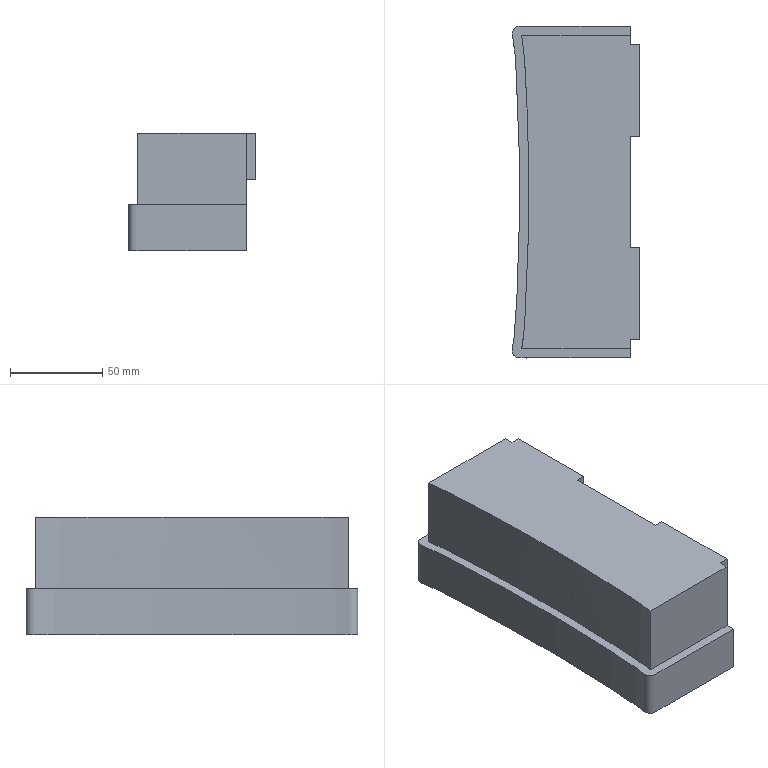Part | NX | features solid 2 | 1 solid | 28 faces | box 69.104 x 180.06 x 64 mm | volume 482191 mm3 | plane 19 | spline 5 | cylinder 4 | commonest cylinder face diameters 20 x2 30 x2
STEP:
#1=CARTESIAN_POINT('',(770.,80.,130.));
#2=VERTEX_POINT('',#1);
#3=CARTESIAN_POINT('',(770.,85.,130.));
#4=VERTEX_POINT('',#3);
#5=CARTESIAN_POINT('',(770.,120.,130.));
#6=DIRECTION('',(0.,-1.,0.));
#7=VECTOR('',#6,1000.);
#8=LINE('',#5,#7);
#9=EDGE_CURVE('',#2,#4,#8,.F.);
#10=ORIENTED_EDGE('',*,*,#9,.F.);
#11=CARTESIAN_POINT('',(770.,80.,105.));
#12=VERTEX_POINT('',#11);
#13=CARTESIAN_POINT('',(770.,80.,130.));
#14=DIRECTION('',(0.,0.,1.));
#15=VECTOR('',#14,1000.);
#16=LINE('',#13,#15);
#17=EDGE_CURVE('',#2,#12,#16,.F.);
#18=ORIENTED_EDGE('',*,*,#17,.T.);
#19=CARTESIAN_POINT('',(770.,65.,105.));
#20=VERTEX_POINT('',#19);
#21=CARTESIAN_POINT('',(770.,50.,105.));
#22=DIRECTION('',(0.,1.,0.));
#23=VECTOR('',#22,1000.);
#24=LINE('',#21,#23);
#25=EDGE_CURVE('',#12,#20,#24,.F.);
#26=ORIENTED_EDGE('',*,*,#25,.T.);
#27=CARTESIAN_POINT('',(770.,65.,66.));
#28=VERTEX_POINT('',#27);
#29=CARTESIAN_POINT('',(770.,65.,50.));
#30=DIRECTION('',(0.,0.,-1.));
#31=VECTOR('',#30,1000.);
#32=LINE('',#29,#31);
#33=EDGE_CURVE('',#28,#20,#32,.F.);
#34=ORIENTED_EDGE('',*,*,#33,.F.);
#35=CARTESIAN_POINT('',(770.,90.,66.));
#36=VERTEX_POINT('',#35);
#37=CARTESIAN_POINT('',(770.,120.,66.));
#38=DIRECTION('',(0.,1.,0.));
#39=VECTOR('',#38,1000.);
#40=LINE('',#37,#39);
#41=EDGE_CURVE('',#36,#28,#40,.F.);
#42=ORIENTED_EDGE('',*,*,#41,.F.);
#43=CARTESIAN_POINT('',(770.,90.,91.));
#44=VERTEX_POINT('',#43);
#45=CARTESIAN_POINT('',(770.,90.,98.));
#46=DIRECTION('',(0.,0.,1.));
#47=VECTOR('',#46,1000.);
#48=LINE('',#45,#47);
#49=EDGE_CURVE('',#36,#44,#48,.T.);
#50=ORIENTED_EDGE('',*,*,#49,.T.);
#51=CARTESIAN_POINT('',(770.,85.,91.));
#52=VERTEX_POINT('',#51);
#53=CARTESIAN_POINT('',(770.,90.,91.));
#54=DIRECTION('',(0.,-1.,0.));
#55=VECTOR('',#54,1000.);
#56=LINE('',#53,#55);
#57=EDGE_CURVE('',#44,#52,#56,.T.);
#58=ORIENTED_EDGE('',*,*,#57,.T.);
#59=CARTESIAN_POINT('',(770.,85.,91.));
#60=DIRECTION('',(0.,0.,1.));
#61=VECTOR('',#60,1000.);
#62=LINE('',#59,#61);
#63=EDGE_CURVE('',#52,#4,#62,.T.);
#64=ORIENTED_EDGE('',*,*,#63,.T.);
#65=EDGE_LOOP('',(#10,#18,#26,#34,#42,#50,#58,#64));
#66=FACE_BOUND('',#65,.T.);
#67=CARTESIAN_POINT('',(770.,120.,50.));
#68=DIRECTION('',(1.,0.,0.));
#69=DIRECTION('',(0.,0.,-1.));
#70=AXIS2_PLACEMENT_3D('',#67,#68,#69);
#71=PLANE('',#70);
#72=ADVANCED_FACE('',(#66),#71,.T.);
#73=CARTESIAN_POINT('',(770.,30.,105.));
#74=VERTEX_POINT('',#73);
#75=CARTESIAN_POINT('',(770.,-30.,105.));
#76=VERTEX_POINT('',#75);
#77=CARTESIAN_POINT('',(770.,120.,105.));
#78=DIRECTION('',(0.,1.,0.));
#79=VECTOR('',#78,1000.);
#80=LINE('',#77,#79);
#81=EDGE_CURVE('',#74,#76,#80,.F.);
#82=ORIENTED_EDGE('',*,*,#81,.F.);
#83=CARTESIAN_POINT('',(770.,30.,130.));
#84=VERTEX_POINT('',#83);
#85=CARTESIAN_POINT('',(770.,30.,130.));
#86=DIRECTION('',(0.,0.,-1.));
#87=VECTOR('',#86,1000.);
#88=LINE('',#85,#87);
#89=EDGE_CURVE('',#84,#74,#88,.T.);
#90=ORIENTED_EDGE('',*,*,#89,.F.);
#91=CARTESIAN_POINT('',(770.,-30.,130.));
#92=VERTEX_POINT('',#91);
#93=CARTESIAN_POINT('',(770.,120.,130.));
#94=DIRECTION('',(0.,-1.,0.));
#95=VECTOR('',#94,1000.);
#96=LINE('',#93,#95);
#97=EDGE_CURVE('',#92,#84,#96,.F.);
#98=ORIENTED_EDGE('',*,*,#97,.F.);
#99=CARTESIAN_POINT('',(770.,-30.,130.));
#100=DIRECTION('',(0.,0.,-1.));
#101=VECTOR('',#100,1000.);
#102=LINE('',#99,#101);
#103=EDGE_CURVE('',#92,#76,#102,.T.);
#104=ORIENTED_EDGE('',*,*,#103,.T.);
#105=EDGE_LOOP('',(#82,#90,#98,#104));
#106=FACE_BOUND('',#105,.T.);
#107=CARTESIAN_POINT('',(770.,120.,50.));
#108=DIRECTION('',(1.,0.,0.));
#109=DIRECTION('',(0.,0.,-1.));
#110=AXIS2_PLACEMENT_3D('',#107,#108,#109);
#111=PLANE('',#110);
#112=ADVANCED_FACE('',(#106),#111,.T.);
#113=CARTESIAN_POINT('',(711.016,85.028,130.));
#114=VERTEX_POINT('',#113);
#115=CARTESIAN_POINT('',(711.009,-85.029,130.));
#116=VERTEX_POINT('',#115);
#117=CARTESIAN_POINT('',(711.016,85.028,130.));
#118=CARTESIAN_POINT('',(711.113,84.38,130.));
#119=CARTESIAN_POINT('',(711.28,83.237,130.));
#120=CARTESIAN_POINT('',(711.512,81.583,130.));
#121=CARTESIAN_POINT('',(711.653,80.568,130.));
#122=CARTESIAN_POINT('',(711.81,79.426,130.));
#123=CARTESIAN_POINT('',(711.951,78.38,130.));
#124=CARTESIAN_POINT('',(712.186,76.65,130.));
#125=CARTESIAN_POINT('',(712.426,74.446,130.));
#126=CARTESIAN_POINT('',(712.563,71.77,130.));
#127=CARTESIAN_POINT('',(712.789,68.223,130.));
#128=CARTESIAN_POINT('',(713.036,63.843,130.));
#129=CARTESIAN_POINT('',(713.326,58.444,130.));
#130=CARTESIAN_POINT('',(713.587,53.129,130.));
#131=CARTESIAN_POINT('',(713.826,47.81,130.));
#132=CARTESIAN_POINT('',(714.036,42.612,130.));
#133=CARTESIAN_POINT('',(714.234,37.124,130.));
#134=CARTESIAN_POINT('',(714.457,29.957,130.));
#135=CARTESIAN_POINT('',(714.674,21.033,130.));
#136=CARTESIAN_POINT('',(714.828,10.445,130.));
#137=CARTESIAN_POINT('',(714.895,-3.481,130.));
#138=CARTESIAN_POINT('',(714.754,-17.426,130.));
#139=CARTESIAN_POINT('',(714.447,-29.939,130.));
#140=CARTESIAN_POINT('',(714.221,-37.113,130.));
#141=CARTESIAN_POINT('',(714.022,-42.617,130.));
#142=CARTESIAN_POINT('',(713.812,-47.802,130.));
#143=CARTESIAN_POINT('',(713.573,-53.121,130.));
#144=CARTESIAN_POINT('',(713.312,-58.436,130.));
#145=CARTESIAN_POINT('',(713.023,-63.845,130.));
#146=CARTESIAN_POINT('',(712.772,-68.224,130.));
#147=CARTESIAN_POINT('',(712.585,-71.32,130.));
#148=CARTESIAN_POINT('',(712.487,-72.892,130.));
#149=CARTESIAN_POINT('',(712.433,-73.755,130.));
#150=CARTESIAN_POINT('',(712.387,-74.507,130.));
#151=CARTESIAN_POINT('',(712.36,-74.864,130.));
#152=CARTESIAN_POINT('',(712.291,-75.607,130.));
#153=CARTESIAN_POINT('',(712.173,-76.66,130.));
#154=CARTESIAN_POINT('',(711.96,-78.303,130.));
#155=CARTESIAN_POINT('',(711.632,-80.652,130.));
#156=CARTESIAN_POINT('',(711.306,-82.996,130.));
#157=CARTESIAN_POINT('',(711.097,-84.435,130.));
#158=CARTESIAN_POINT('',(711.009,-85.029,130.));
#159=B_SPLINE_CURVE_WITH_KNOTS('',3,(#117,#118,#119,#120,#121,#122,#123,#124,#125,#126,#127,#128,#129,#130,#131,#132,#133,#134,#135,#136,#137,#138,#139,#140,#141,#142,#143,#144,#145,#146,#147,#148,#149,#150,#151,#152,#153,#154,#155,#156,#157,#158),.UNSPECIFIED.,.F.,.F.,(4,1,1,1,1,1,1,1,1,1,1,1,1,1,1,1,1,1,1,1,1,1,1,1,1,1,1,1,1,1,1,1,1,1,1,1,1,1,1,4),(0.,0.01562,0.02344,0.02734,0.03125,0.03906,0.04688,0.0625,0.07812,0.09375,0.125,0.1562,0.1875,0.2188,0.25,0.2812,0.3125,0.375,0.4375,0.5,0.625,0.6875,0.7188,0.75,0.7812,0.8125,0.8438,0.875,0.9062,0.9219,0.9297,0.9336,0.9375,0.9414,0.9453,0.9531,0.9609,0.9688,0.9844,1.),.UNSPECIFIED.);
#160=EDGE_CURVE('',#114,#116,#159,.T.);
#161=ORIENTED_EDGE('',*,*,#160,.T.);
#162=CARTESIAN_POINT('',(770.,-85.,130.));
#163=VERTEX_POINT('',#162);
#164=CARTESIAN_POINT('',(711.009,-85.029,130.));
#165=CARTESIAN_POINT('',(717.1,-85.01,130.));
#166=CARTESIAN_POINT('',(736.764,-85.,130.));
#167=CARTESIAN_POINT('',(770.,-85.,130.));
#168=B_SPLINE_CURVE_WITH_KNOTS('',3,(#164,#165,#166,#167),.UNSPECIFIED.,.F.,.F.,(4,4),(0.,1.),.UNSPECIFIED.);
#169=EDGE_CURVE('',#116,#163,#168,.T.);
#170=ORIENTED_EDGE('',*,*,#169,.T.);
#171=CARTESIAN_POINT('',(770.,-80.,130.));
#172=VERTEX_POINT('',#171);
#173=CARTESIAN_POINT('',(770.,120.,130.));
#174=DIRECTION('',(0.,-1.,0.));
#175=VECTOR('',#174,1000.);
#176=LINE('',#173,#175);
#177=EDGE_CURVE('',#163,#172,#176,.F.);
#178=ORIENTED_EDGE('',*,*,#177,.T.);
#179=CARTESIAN_POINT('',(775.,-80.,130.));
#180=VERTEX_POINT('',#179);
#181=CARTESIAN_POINT('',(775.,-80.,130.));
#182=DIRECTION('',(-1.,0.,0.));
#183=VECTOR('',#182,1000.);
#184=LINE('',#181,#183);
#185=EDGE_CURVE('',#180,#172,#184,.T.);
#186=ORIENTED_EDGE('',*,*,#185,.F.);
#187=CARTESIAN_POINT('',(775.,-30.,130.));
#188=VERTEX_POINT('',#187);
#189=CARTESIAN_POINT('',(775.,-90.,130.));
#190=DIRECTION('',(0.,1.,0.));
#191=VECTOR('',#190,1000.);
#192=LINE('',#189,#191);
#193=EDGE_CURVE('',#180,#188,#192,.T.);
#194=ORIENTED_EDGE('',*,*,#193,.T.);
#195=CARTESIAN_POINT('',(775.,-30.,130.));
#196=DIRECTION('',(-1.,0.,0.));
#197=VECTOR('',#196,1000.);
#198=LINE('',#195,#197);
#199=EDGE_CURVE('',#188,#92,#198,.T.);
#200=ORIENTED_EDGE('',*,*,#199,.T.);
#201=ORIENTED_EDGE('',*,*,#97,.T.);
#202=CARTESIAN_POINT('',(775.,30.,130.));
#203=VERTEX_POINT('',#202);
#204=CARTESIAN_POINT('',(775.,30.,130.));
#205=DIRECTION('',(-1.,0.,0.));
#206=VECTOR('',#205,1000.);
#207=LINE('',#204,#206);
#208=EDGE_CURVE('',#203,#84,#207,.T.);
#209=ORIENTED_EDGE('',*,*,#208,.F.);
#210=CARTESIAN_POINT('',(775.,80.,130.));
#211=VERTEX_POINT('',#210);
#212=CARTESIAN_POINT('',(775.,50.,130.));
#213=DIRECTION('',(0.,-1.,0.));
#214=VECTOR('',#213,1000.);
#215=LINE('',#212,#214);
#216=EDGE_CURVE('',#211,#203,#215,.T.);
#217=ORIENTED_EDGE('',*,*,#216,.F.);
#218=CARTESIAN_POINT('',(775.,80.,130.));
#219=DIRECTION('',(1.,0.,0.));
#220=VECTOR('',#219,1000.);
#221=LINE('',#218,#220);
#222=EDGE_CURVE('',#211,#2,#221,.F.);
#223=ORIENTED_EDGE('',*,*,#222,.T.);
#224=ORIENTED_EDGE('',*,*,#9,.T.);
#225=CARTESIAN_POINT('',(770.,85.,130.));
#226=CARTESIAN_POINT('',(735.052,85.,130.));
#227=CARTESIAN_POINT('',(715.391,85.009,130.));
#228=CARTESIAN_POINT('',(711.016,85.028,130.));
#229=B_SPLINE_CURVE_WITH_KNOTS('',3,(#225,#226,#227,#228),.UNSPECIFIED.,.F.,.F.,(4,4),(0.,1.),.UNSPECIFIED.);
#230=EDGE_CURVE('',#4,#114,#229,.T.);
#231=ORIENTED_EDGE('',*,*,#230,.T.);
#232=EDGE_LOOP('',(#161,#170,#178,#186,#194,#200,#201,#209,#217,#223,#224,#231));
#233=FACE_BOUND('',#232,.T.);
#234=CARTESIAN_POINT('',(0.,0.,130.));
#235=DIRECTION('',(0.,0.,1.));
#236=DIRECTION('',(1.,0.,0.));
#237=AXIS2_PLACEMENT_3D('',#234,#235,#236);
#238=PLANE('',#237);
#239=ADVANCED_FACE('',(#233),#238,.T.);
#240=CARTESIAN_POINT('',(770.,-90.,91.));
#241=VERTEX_POINT('',#240);
#242=CARTESIAN_POINT('',(770.,-90.,66.));
#243=VERTEX_POINT('',#242);
#244=CARTESIAN_POINT('',(770.,-90.,98.));
#245=DIRECTION('',(0.,0.,1.));
#246=VECTOR('',#245,1000.);
#247=LINE('',#244,#246);
#248=EDGE_CURVE('',#241,#243,#247,.F.);
#249=ORIENTED_EDGE('',*,*,#248,.F.);
#250=CARTESIAN_POINT('',(790.,-90.,91.));
#251=CARTESIAN_POINT('',(782.313,-90.,91.));
#252=CARTESIAN_POINT('',(774.625,-90.,91.));
#253=CARTESIAN_POINT('',(766.938,-90.,91.));
#254=CARTESIAN_POINT('',(757.429,-90.,91.));
#255=CARTESIAN_POINT('',(738.707,-90.,91.));
#256=CARTESIAN_POINT('',(719.689,-90.,91.));
#257=CARTESIAN_POINT('',(709.611,-90.034,91.));
#258=CARTESIAN_POINT('',(708.18,-89.742,91.));
#259=CARTESIAN_POINT('',(706.773,-88.715,91.));
#260=CARTESIAN_POINT('',(705.945,-87.182,91.));
#261=CARTESIAN_POINT('',(705.849,-85.71,91.));
#262=CARTESIAN_POINT('',(706.186,-83.502,91.));
#263=CARTESIAN_POINT('',(706.636,-80.205,91.));
#264=CARTESIAN_POINT('',(707.096,-77.043,91.));
#265=CARTESIAN_POINT('',(707.332,-75.034,91.));
#266=CARTESIAN_POINT('',(707.37,-74.599,91.));
#267=CARTESIAN_POINT('',(708.17,-62.019,91.));
#268=CARTESIAN_POINT('',(709.408,-37.195,91.));
#269=CARTESIAN_POINT('',(710.084,-0.0009582,91.));
#270=CARTESIAN_POINT('',(709.422,37.194,91.));
#271=CARTESIAN_POINT('',(708.185,62.018,91.));
#272=CARTESIAN_POINT('',(707.381,74.598,91.));
#273=CARTESIAN_POINT('',(707.346,75.035,91.));
#274=CARTESIAN_POINT('',(707.091,77.042,91.));
#275=CARTESIAN_POINT('',(706.658,80.207,91.));
#276=CARTESIAN_POINT('',(706.194,83.501,91.));
#277=CARTESIAN_POINT('',(705.854,85.708,91.));
#278=CARTESIAN_POINT('',(705.949,87.18,91.));
#279=CARTESIAN_POINT('',(706.777,88.714,91.));
#280=CARTESIAN_POINT('',(708.184,89.742,91.));
#281=CARTESIAN_POINT('',(709.621,90.034,91.));
#282=CARTESIAN_POINT('',(717.126,90.,91.));
#283=CARTESIAN_POINT('',(730.996,90.,91.));
#284=CARTESIAN_POINT('',(744.562,90.,91.));
#285=CARTESIAN_POINT('',(751.497,90.,91.));
#286=CARTESIAN_POINT('',(764.331,90.,91.));
#287=CARTESIAN_POINT('',(777.166,90.,91.));
#288=CARTESIAN_POINT('',(790.,90.,91.));
#289=B_SPLINE_CURVE_WITH_KNOTS('',3,(#250,#251,#252,#253,#254,#255,#256,#257,#258,#259,#260,#261,#262,#263,#264,#265,#266,#267,#268,#269,#270,#271,#272,#273,#274,#275,#276,#277,#278,#279,#280,#281,#282,#283,#284,#285,#286,#287,#288),.UNSPECIFIED.,.F.,.F.,(4,3,1,1,1,1,1,1,1,1,1,1,1,1,1,1,1,1,1,1,1,1,1,1,1,1,1,1,1,1,1,3,4),(-0.08134,0.,0.1006,0.1981,0.2012,0.2072,0.2133,0.2193,0.2253,0.2286,0.2429,0.2605,0.2624,0.2643,0.2651,0.3958,0.5272,0.6587,0.7893,0.7902,0.7921,0.794,0.8116,0.8259,0.8292,0.8352,0.8412,0.8472,0.8532,0.8565,0.9266,1.,1.136),.UNSPECIFIED.);
#290=EDGE_CURVE('',#241,#44,#289,.T.);
#291=ORIENTED_EDGE('',*,*,#290,.T.);
#292=ORIENTED_EDGE('',*,*,#49,.F.);
#293=CARTESIAN_POINT('',(809.468,-90.,66.));
#294=CARTESIAN_POINT('',(795.291,-90.,66.));
#295=CARTESIAN_POINT('',(781.115,-90.,66.));
#296=CARTESIAN_POINT('',(766.938,-90.,66.));
#297=CARTESIAN_POINT('',(757.429,-90.,66.));
#298=CARTESIAN_POINT('',(738.707,-90.,66.));
#299=CARTESIAN_POINT('',(719.689,-90.,66.));
#300=CARTESIAN_POINT('',(709.611,-90.034,66.));
#301=CARTESIAN_POINT('',(708.18,-89.742,66.));
#302=CARTESIAN_POINT('',(706.773,-88.715,66.));
#303=CARTESIAN_POINT('',(705.945,-87.182,66.));
#304=CARTESIAN_POINT('',(705.849,-85.71,66.));
#305=CARTESIAN_POINT('',(706.186,-83.502,66.));
#306=CARTESIAN_POINT('',(706.636,-80.205,66.));
#307=CARTESIAN_POINT('',(707.096,-77.043,66.));
#308=CARTESIAN_POINT('',(707.332,-75.034,66.));
#309=CARTESIAN_POINT('',(707.37,-74.599,66.));
#310=CARTESIAN_POINT('',(708.17,-62.019,66.));
#311=CARTESIAN_POINT('',(709.408,-37.195,66.));
#312=CARTESIAN_POINT('',(710.084,-0.0009582,66.));
#313=CARTESIAN_POINT('',(709.422,37.194,66.));
#314=CARTESIAN_POINT('',(708.185,62.018,66.));
#315=CARTESIAN_POINT('',(707.381,74.598,66.));
#316=CARTESIAN_POINT('',(707.346,75.035,66.));
#317=CARTESIAN_POINT('',(707.091,77.042,66.));
#318=CARTESIAN_POINT('',(706.658,80.207,66.));
#319=CARTESIAN_POINT('',(706.194,83.501,66.));
#320=CARTESIAN_POINT('',(705.854,85.708,66.));
#321=CARTESIAN_POINT('',(705.949,87.18,66.));
#322=CARTESIAN_POINT('',(706.777,88.714,66.));
#323=CARTESIAN_POINT('',(708.184,89.742,66.));
#324=CARTESIAN_POINT('',(709.621,90.034,66.));
#325=CARTESIAN_POINT('',(717.126,90.,66.));
#326=CARTESIAN_POINT('',(730.996,90.,66.));
#327=CARTESIAN_POINT('',(744.562,90.,66.));
#328=CARTESIAN_POINT('',(751.497,90.,66.));
#329=CARTESIAN_POINT('',(765.674,90.,66.));
#330=CARTESIAN_POINT('',(779.851,90.,66.));
#331=CARTESIAN_POINT('',(794.028,90.,66.));
#332=B_SPLINE_CURVE_WITH_KNOTS('',3,(#293,#294,#295,#296,#297,#298,#299,#300,#301,#302,#303,#304,#305,#306,#307,#308,#309,#310,#311,#312,#313,#314,#315,#316,#317,#318,#319,#320,#321,#322,#323,#324,#325,#326,#327,#328,#329,#330,#331),.UNSPECIFIED.,.F.,.F.,(4,3,1,1,1,1,1,1,1,1,1,1,1,1,1,1,1,1,1,1,1,1,1,1,1,1,1,1,1,1,1,3,4),(-0.15,0.,0.1006,0.1981,0.2012,0.2072,0.2133,0.2193,0.2253,0.2286,0.2429,0.2605,0.2624,0.2643,0.2651,0.3958,0.5272,0.6587,0.7893,0.7902,0.7921,0.794,0.8116,0.8259,0.8292,0.8352,0.8412,0.8472,0.8532,0.8565,0.9266,1.,1.15),.UNSPECIFIED.);
#333=EDGE_CURVE('',#36,#243,#332,.F.);
#334=ORIENTED_EDGE('',*,*,#333,.T.);
#335=EDGE_LOOP('',(#249,#291,#292,#334));
#336=FACE_BOUND('',#335,.T.);
#337=CARTESIAN_POINT('',(770.,-90.,66.));
#338=CARTESIAN_POINT('',(770.,-90.,91.));
#339=CARTESIAN_POINT('',(768.979,-90.,66.));
#340=CARTESIAN_POINT('',(768.979,-90.,91.));
#341=CARTESIAN_POINT('',(767.958,-90.,66.));
#342=CARTESIAN_POINT('',(767.958,-90.,91.));
#343=CARTESIAN_POINT('',(766.938,-90.,66.));
#344=CARTESIAN_POINT('',(766.938,-90.,91.));
#345=CARTESIAN_POINT('',(757.429,-90.,66.));
#346=CARTESIAN_POINT('',(757.429,-90.,91.));
#347=CARTESIAN_POINT('',(738.707,-90.,66.));
#348=CARTESIAN_POINT('',(738.707,-90.,91.));
#349=CARTESIAN_POINT('',(719.689,-90.,66.));
#350=CARTESIAN_POINT('',(719.689,-90.,91.));
#351=CARTESIAN_POINT('',(709.611,-90.034,66.));
#352=CARTESIAN_POINT('',(709.611,-90.034,91.));
#353=CARTESIAN_POINT('',(708.18,-89.742,66.));
#354=CARTESIAN_POINT('',(708.18,-89.742,91.));
#355=CARTESIAN_POINT('',(706.773,-88.715,66.));
#356=CARTESIAN_POINT('',(706.773,-88.715,91.));
#357=CARTESIAN_POINT('',(705.945,-87.182,66.));
#358=CARTESIAN_POINT('',(705.945,-87.182,91.));
#359=CARTESIAN_POINT('',(705.849,-85.71,66.));
#360=CARTESIAN_POINT('',(705.849,-85.71,91.));
#361=CARTESIAN_POINT('',(706.186,-83.502,66.));
#362=CARTESIAN_POINT('',(706.186,-83.502,91.));
#363=CARTESIAN_POINT('',(706.636,-80.205,66.));
#364=CARTESIAN_POINT('',(706.636,-80.205,91.));
#365=CARTESIAN_POINT('',(707.096,-77.043,66.));
#366=CARTESIAN_POINT('',(707.096,-77.043,91.));
#367=CARTESIAN_POINT('',(707.332,-75.034,66.));
#368=CARTESIAN_POINT('',(707.332,-75.034,91.));
#369=CARTESIAN_POINT('',(707.37,-74.599,66.));
#370=CARTESIAN_POINT('',(707.37,-74.599,91.));
#371=CARTESIAN_POINT('',(708.17,-62.019,66.));
#372=CARTESIAN_POINT('',(708.17,-62.019,91.));
#373=CARTESIAN_POINT('',(709.408,-37.195,66.));
#374=CARTESIAN_POINT('',(709.408,-37.195,91.));
#375=CARTESIAN_POINT('',(710.084,-0.0009582,66.));
#376=CARTESIAN_POINT('',(710.084,-0.0009582,91.));
#377=CARTESIAN_POINT('',(709.422,37.194,66.));
#378=CARTESIAN_POINT('',(709.422,37.194,91.));
#379=CARTESIAN_POINT('',(708.185,62.018,66.));
#380=CARTESIAN_POINT('',(708.185,62.018,91.));
#381=CARTESIAN_POINT('',(707.381,74.598,66.));
#382=CARTESIAN_POINT('',(707.381,74.598,91.));
#383=CARTESIAN_POINT('',(707.346,75.035,66.));
#384=CARTESIAN_POINT('',(707.346,75.035,91.));
#385=CARTESIAN_POINT('',(707.091,77.042,66.));
#386=CARTESIAN_POINT('',(707.091,77.042,91.));
#387=CARTESIAN_POINT('',(706.658,80.207,66.));
#388=CARTESIAN_POINT('',(706.658,80.207,91.));
#389=CARTESIAN_POINT('',(706.194,83.501,66.));
#390=CARTESIAN_POINT('',(706.194,83.501,91.));
#391=CARTESIAN_POINT('',(705.854,85.708,66.));
#392=CARTESIAN_POINT('',(705.854,85.708,91.));
#393=CARTESIAN_POINT('',(705.949,87.18,66.));
#394=CARTESIAN_POINT('',(705.949,87.18,91.));
#395=CARTESIAN_POINT('',(706.777,88.714,66.));
#396=CARTESIAN_POINT('',(706.777,88.714,91.));
#397=CARTESIAN_POINT('',(708.184,89.742,66.));
#398=CARTESIAN_POINT('',(708.184,89.742,91.));
#399=CARTESIAN_POINT('',(709.621,90.034,66.));
#400=CARTESIAN_POINT('',(709.621,90.034,91.));
#401=CARTESIAN_POINT('',(717.126,90.,66.));
#402=CARTESIAN_POINT('',(717.126,90.,91.));
#403=CARTESIAN_POINT('',(730.996,90.,66.));
#404=CARTESIAN_POINT('',(730.996,90.,91.));
#405=CARTESIAN_POINT('',(744.562,90.,66.));
#406=CARTESIAN_POINT('',(744.562,90.,91.));
#407=CARTESIAN_POINT('',(751.497,90.,66.));
#408=CARTESIAN_POINT('',(751.497,90.,91.));
#409=CARTESIAN_POINT('',(757.665,90.,66.));
#410=CARTESIAN_POINT('',(757.665,90.,91.));
#411=CARTESIAN_POINT('',(763.832,90.,66.));
#412=CARTESIAN_POINT('',(763.832,90.,91.));
#413=CARTESIAN_POINT('',(770.,90.,66.));
#414=CARTESIAN_POINT('',(770.,90.,91.));
#415=B_SPLINE_SURFACE_WITH_KNOTS('',3,1,((#337,#338),(#339,#340),(#341,#342),(#343,#344),(#345,#346),(#347,#348),(#349,#350),(#351,#352),(#353,#354),(#355,#356),(#357,#358),(#359,#360),(#361,#362),(#363,#364),(#365,#366),(#367,#368),(#369,#370),(#371,#372),(#373,#374),(#375,#376),(#377,#378),(#379,#380),(#381,#382),(#383,#384),(#385,#386),(#387,#388),(#389,#390),(#391,#392),(#393,#394),(#395,#396),(#397,#398),(#399,#400),(#401,#402),(#403,#404),(#405,#406),(#407,#408),(#409,#410),(#411,#412),(#413,#414)),.SURF_OF_LINEAR_EXTRUSION.,.F.,.F.,.F.,(4,3,1,1,1,1,1,1,1,1,1,1,1,1,1,1,1,1,1,1,1,1,1,1,1,1,1,1,1,1,1,3,4),(2,2),(-0.0108,0.,0.1006,0.1981,0.2012,0.2072,0.2133,0.2193,0.2253,0.2286,0.2429,0.2605,0.2624,0.2643,0.2651,0.3958,0.5272,0.6587,0.7893,0.7902,0.7921,0.794,0.8116,0.8259,0.8292,0.8352,0.8412,0.8472,0.8532,0.8565,0.9266,1.,1.065),(0.,1.),.UNSPECIFIED.);
#416=ADVANCED_FACE('',(#336),#415,.F.);
#417=CARTESIAN_POINT('',(770.,-65.,66.));
#418=VERTEX_POINT('',#417);
#419=CARTESIAN_POINT('',(770.,-65.,105.));
#420=VERTEX_POINT('',#419);
#421=CARTESIAN_POINT('',(770.,-65.,50.));
#422=DIRECTION('',(0.,0.,-1.));
#423=VECTOR('',#422,1000.);
#424=LINE('',#421,#423);
#425=EDGE_CURVE('',#418,#420,#424,.F.);
#426=ORIENTED_EDGE('',*,*,#425,.T.);
#427=CARTESIAN_POINT('',(770.,-80.,105.));
#428=VERTEX_POINT('',#427);
#429=CARTESIAN_POINT('',(770.,-90.,105.));
#430=DIRECTION('',(0.,1.,0.));
#431=VECTOR('',#430,1000.);
#432=LINE('',#429,#431);
#433=EDGE_CURVE('',#428,#420,#432,.T.);
#434=ORIENTED_EDGE('',*,*,#433,.F.);
#435=CARTESIAN_POINT('',(770.,-80.,130.));
#436=DIRECTION('',(0.,0.,-1.));
#437=VECTOR('',#436,1000.);
#438=LINE('',#435,#437);
#439=EDGE_CURVE('',#172,#428,#438,.T.);
#440=ORIENTED_EDGE('',*,*,#439,.F.);
#441=ORIENTED_EDGE('',*,*,#177,.F.);
#442=CARTESIAN_POINT('',(770.,-85.,91.));
#443=VERTEX_POINT('',#442);
#444=CARTESIAN_POINT('',(770.,-85.,91.));
#445=DIRECTION('',(0.,0.,1.));
#446=VECTOR('',#445,1000.);
#447=LINE('',#444,#446);
#448=EDGE_CURVE('',#443,#163,#447,.T.);
#449=ORIENTED_EDGE('',*,*,#448,.F.);
#450=CARTESIAN_POINT('',(770.,-90.,91.));
#451=DIRECTION('',(0.,1.,0.));
#452=VECTOR('',#451,1000.);
#453=LINE('',#450,#452);
#454=EDGE_CURVE('',#241,#443,#453,.T.);
#455=ORIENTED_EDGE('',*,*,#454,.F.);
#456=ORIENTED_EDGE('',*,*,#248,.T.);
#457=CARTESIAN_POINT('',(770.,120.,66.));
#458=DIRECTION('',(0.,1.,0.));
#459=VECTOR('',#458,1000.);
#460=LINE('',#457,#459);
#461=EDGE_CURVE('',#418,#243,#460,.F.);
#462=ORIENTED_EDGE('',*,*,#461,.F.);
#463=EDGE_LOOP('',(#426,#434,#440,#441,#449,#455,#456,#462));
#464=FACE_BOUND('',#463,.T.);
#465=CARTESIAN_POINT('',(770.,120.,50.));
#466=DIRECTION('',(1.,0.,0.));
#467=DIRECTION('',(0.,0.,-1.));
#468=AXIS2_PLACEMENT_3D('',#465,#466,#467);
#469=PLANE('',#468);
#470=ADVANCED_FACE('',(#464),#469,.T.);
#471=CARTESIAN_POINT('',(751.497,65.,105.));
#472=VERTEX_POINT('',#471);
#473=CARTESIAN_POINT('',(820.,65.,105.));
#474=DIRECTION('',(-1.,0.,0.));
#475=VECTOR('',#474,1000.);
#476=LINE('',#473,#475);
#477=EDGE_CURVE('',#20,#472,#476,.T.);
#478=ORIENTED_EDGE('',*,*,#477,.T.);
#479=CARTESIAN_POINT('',(751.497,65.,66.));
#480=VERTEX_POINT('',#479);
#481=CARTESIAN_POINT('',(751.497,65.,37.));
#482=DIRECTION('',(0.,0.,1.));
#483=VECTOR('',#482,1000.);
#484=LINE('',#481,#483);
#485=EDGE_CURVE('',#480,#472,#484,.T.);
#486=ORIENTED_EDGE('',*,*,#485,.F.);
#487=CARTESIAN_POINT('',(820.,65.,66.));
#488=DIRECTION('',(-1.,0.,0.));
#489=VECTOR('',#488,1000.);
#490=LINE('',#487,#489);
#491=EDGE_CURVE('',#28,#480,#490,.T.);
#492=ORIENTED_EDGE('',*,*,#491,.F.);
#493=ORIENTED_EDGE('',*,*,#33,.T.);
#494=EDGE_LOOP('',(#478,#486,#492,#493));
#495=FACE_BOUND('',#494,.T.);
#496=CARTESIAN_POINT('',(751.497,65.,37.));
#497=DIRECTION('',(0.,-1.,0.));
#498=DIRECTION('',(1.,0.,0.));
#499=AXIS2_PLACEMENT_3D('',#496,#497,#498);
#500=PLANE('',#499);
#501=ADVANCED_FACE('',(#495),#500,.T.);
#502=CARTESIAN_POINT('',(766.938,-65.,105.));
#503=VERTEX_POINT('',#502);
#504=CARTESIAN_POINT('',(751.497,65.,105.));
#505=CARTESIAN_POINT('',(750.645,64.603,105.));
#506=CARTESIAN_POINT('',(748.739,64.254,105.));
#507=CARTESIAN_POINT('',(745.971,64.398,105.));
#508=CARTESIAN_POINT('',(743.186,64.831,105.));
#509=CARTESIAN_POINT('',(740.429,65.377,105.));
#510=CARTESIAN_POINT('',(738.115,65.792,105.));
#511=CARTESIAN_POINT('',(736.253,65.947,105.));
#512=CARTESIAN_POINT('',(734.844,65.888,105.));
#513=CARTESIAN_POINT('',(733.457,65.414,105.));
#514=CARTESIAN_POINT('',(732.64,64.182,105.));
#515=CARTESIAN_POINT('',(732.485,62.764,105.));
#516=CARTESIAN_POINT('',(732.592,60.909,105.));
#517=CARTESIAN_POINT('',(733.01,58.592,105.));
#518=CARTESIAN_POINT('',(733.725,54.911,105.));
#519=CARTESIAN_POINT('',(734.,51.164,105.));
#520=CARTESIAN_POINT('',(733.823,47.38,105.));
#521=CARTESIAN_POINT('',(733.811,43.604,105.));
#522=CARTESIAN_POINT('',(734.18,38.888,105.));
#523=CARTESIAN_POINT('',(734.453,33.225,105.));
#524=CARTESIAN_POINT('',(734.467,27.554,105.));
#525=CARTESIAN_POINT('',(734.617,21.884,105.));
#526=CARTESIAN_POINT('',(734.789,14.324,105.));
#527=CARTESIAN_POINT('',(734.86,4.873,105.));
#528=CARTESIAN_POINT('',(734.838,-6.468,105.));
#529=CARTESIAN_POINT('',(734.744,-15.92,105.));
#530=CARTESIAN_POINT('',(734.573,-23.481,105.));
#531=CARTESIAN_POINT('',(734.511,-29.153,105.));
#532=CARTESIAN_POINT('',(734.334,-34.822,105.));
#533=CARTESIAN_POINT('',(733.931,-40.484,105.));
#534=CARTESIAN_POINT('',(733.951,-45.213,105.));
#535=CARTESIAN_POINT('',(733.978,-48.996,105.));
#536=CARTESIAN_POINT('',(733.78,-51.827,105.));
#537=CARTESIAN_POINT('',(733.378,-54.653,105.));
#538=CARTESIAN_POINT('',(732.915,-57.463,105.));
#539=CARTESIAN_POINT('',(732.66,-59.84,105.));
#540=CARTESIAN_POINT('',(732.806,-61.723,105.));
#541=CARTESIAN_POINT('',(733.299,-63.11,105.));
#542=CARTESIAN_POINT('',(734.37,-64.124,105.));
#543=CARTESIAN_POINT('',(736.185,-64.808,105.));
#544=CARTESIAN_POINT('',(738.548,-65.006,105.));
#545=CARTESIAN_POINT('',(741.382,-65.017,105.));
#546=CARTESIAN_POINT('',(745.17,-64.98,105.));
#547=CARTESIAN_POINT('',(749.901,-65.012,105.));
#548=CARTESIAN_POINT('',(755.58,-65.012,105.));
#549=CARTESIAN_POINT('',(761.259,-64.985,105.));
#550=CARTESIAN_POINT('',(765.045,-64.991,105.));
#551=CARTESIAN_POINT('',(766.938,-65.,105.));
#552=B_SPLINE_CURVE_WITH_KNOTS('',3,(#504,#505,#506,#507,#508,#509,#510,#511,#512,#513,#514,#515,#516,#517,#518,#519,#520,#521,#522,#523,#524,#525,#526,#527,#528,#529,#530,#531,#532,#533,#534,#535,#536,#537,#538,#539,#540,#541,#542,#543,#544,#545,#546,#547,#548,#549,#550,#551),.UNSPECIFIED.,.F.,.F.,(4,1,1,1,1,1,1,1,1,1,1,1,1,1,1,1,1,1,1,1,1,1,1,1,1,1,1,1,1,1,1,1,1,1,1,1,1,1,1,1,1,1,1,1,1,4),(0.1721,0.1749,0.1777,0.1805,0.1833,0.1862,0.1876,0.189,0.1904,0.1918,0.1932,0.1946,0.1974,0.2003,0.2059,0.2087,0.2116,0.2172,0.2228,0.2285,0.2341,0.2398,0.251,0.2623,0.2736,0.2793,0.2849,0.2905,0.2962,0.3018,0.3046,0.3075,0.3103,0.3131,0.3159,0.3173,0.3188,0.3202,0.3216,0.3244,0.3272,0.33,0.3357,0.3413,0.347,0.3526),.UNSPECIFIED.);
#553=EDGE_CURVE('',#472,#503,#552,.T.);
#554=ORIENTED_EDGE('',*,*,#553,.T.);
#555=CARTESIAN_POINT('',(766.938,-65.,66.));
#556=VERTEX_POINT('',#555);
#557=CARTESIAN_POINT('',(766.938,-65.,37.));
#558=DIRECTION('',(0.,0.,1.));
#559=VECTOR('',#558,1000.);
#560=LINE('',#557,#559);
#561=EDGE_CURVE('',#556,#503,#560,.T.);
#562=ORIENTED_EDGE('',*,*,#561,.F.);
#563=CARTESIAN_POINT('',(751.497,65.,66.));
#564=CARTESIAN_POINT('',(750.634,64.597,66.));
#565=CARTESIAN_POINT('',(748.75,64.257,66.));
#566=CARTESIAN_POINT('',(745.957,64.398,66.));
#567=CARTESIAN_POINT('',(743.174,64.834,66.));
#568=CARTESIAN_POINT('',(740.414,65.38,66.));
#569=CARTESIAN_POINT('',(738.099,65.795,66.));
#570=CARTESIAN_POINT('',(736.236,65.948,66.));
#571=CARTESIAN_POINT('',(734.826,65.886,66.));
#572=CARTESIAN_POINT('',(733.44,65.402,66.));
#573=CARTESIAN_POINT('',(732.635,64.162,66.));
#574=CARTESIAN_POINT('',(732.485,62.743,66.));
#575=CARTESIAN_POINT('',(732.596,60.886,66.));
#576=CARTESIAN_POINT('',(733.015,58.568,66.));
#577=CARTESIAN_POINT('',(733.73,54.883,66.));
#578=CARTESIAN_POINT('',(734.,51.134,66.));
#579=CARTESIAN_POINT('',(733.822,47.346,66.));
#580=CARTESIAN_POINT('',(733.812,43.567,66.));
#581=CARTESIAN_POINT('',(734.184,38.848,66.));
#582=CARTESIAN_POINT('',(734.453,33.182,66.));
#583=CARTESIAN_POINT('',(734.468,27.513,66.));
#584=CARTESIAN_POINT('',(734.618,21.845,66.));
#585=CARTESIAN_POINT('',(734.789,14.288,66.));
#586=CARTESIAN_POINT('',(734.86,4.839,66.));
#587=CARTESIAN_POINT('',(734.838,-6.501,66.));
#588=CARTESIAN_POINT('',(734.743,-15.952,66.));
#589=CARTESIAN_POINT('',(734.572,-23.51,66.));
#590=CARTESIAN_POINT('',(734.51,-29.181,66.));
#591=CARTESIAN_POINT('',(734.332,-34.848,66.));
#592=CARTESIAN_POINT('',(733.93,-40.508,66.));
#593=CARTESIAN_POINT('',(733.952,-45.233,66.));
#594=CARTESIAN_POINT('',(733.977,-49.012,66.));
#595=CARTESIAN_POINT('',(733.779,-51.835,66.));
#596=CARTESIAN_POINT('',(733.379,-54.647,66.));
#597=CARTESIAN_POINT('',(732.918,-57.441,66.));
#598=CARTESIAN_POINT('',(732.663,-59.808,66.));
#599=CARTESIAN_POINT('',(732.798,-61.674,66.));
#600=CARTESIAN_POINT('',(733.271,-63.062,66.));
#601=CARTESIAN_POINT('',(734.318,-64.094,66.));
#602=CARTESIAN_POINT('',(736.122,-64.798,66.));
#603=CARTESIAN_POINT('',(738.5,-65.005,66.));
#604=CARTESIAN_POINT('',(741.336,-65.017,66.));
#605=CARTESIAN_POINT('',(745.131,-64.98,66.));
#606=CARTESIAN_POINT('',(749.871,-65.011,66.));
#607=CARTESIAN_POINT('',(755.56,-65.012,66.));
#608=CARTESIAN_POINT('',(761.249,-64.985,66.));
#609=CARTESIAN_POINT('',(765.041,-64.991,66.));
#610=CARTESIAN_POINT('',(766.938,-65.,66.));
#611=B_SPLINE_CURVE_WITH_KNOTS('',3,(#563,#564,#565,#566,#567,#568,#569,#570,#571,#572,#573,#574,#575,#576,#577,#578,#579,#580,#581,#582,#583,#584,#585,#586,#587,#588,#589,#590,#591,#592,#593,#594,#595,#596,#597,#598,#599,#600,#601,#602,#603,#604,#605,#606,#607,#608,#609,#610),.UNSPECIFIED.,.F.,.F.,(4,1,1,1,1,1,1,1,1,1,1,1,1,1,1,1,1,1,1,1,1,1,1,1,1,1,1,1,1,1,1,1,1,1,1,1,1,1,1,1,1,1,1,1,1,4),(0.,0.00282,0.00564,0.008461,0.01128,0.0141,0.01551,0.01692,0.01833,0.01974,0.02115,0.02256,0.02538,0.0282,0.03384,0.03666,0.03948,0.04512,0.05076,0.0564,0.06204,0.06769,0.07897,0.09025,0.1015,0.1072,0.1128,0.1184,0.1241,0.1297,0.1325,0.1354,0.1382,0.141,0.1438,0.1452,0.1467,0.1481,0.1495,0.1523,0.1551,0.1579,0.1636,0.1692,0.1749,0.1805),.UNSPECIFIED.);
#612=EDGE_CURVE('',#480,#556,#611,.T.);
#613=ORIENTED_EDGE('',*,*,#612,.F.);
#614=ORIENTED_EDGE('',*,*,#485,.T.);
#615=EDGE_LOOP('',(#554,#562,#613,#614));
#616=FACE_BOUND('',#615,.T.);
#617=CARTESIAN_POINT('',(766.938,-65.,66.));
#618=CARTESIAN_POINT('',(766.938,-65.,105.));
#619=CARTESIAN_POINT('',(765.045,-64.991,66.));
#620=CARTESIAN_POINT('',(765.045,-64.991,105.));
#621=CARTESIAN_POINT('',(761.247,-64.985,66.));
#622=CARTESIAN_POINT('',(761.247,-64.985,105.));
#623=CARTESIAN_POINT('',(755.515,-65.011,66.));
#624=CARTESIAN_POINT('',(755.515,-65.011,105.));
#625=CARTESIAN_POINT('',(749.805,-65.015,66.));
#626=CARTESIAN_POINT('',(749.805,-65.015,105.));
#627=CARTESIAN_POINT('',(744.157,-64.958,66.));
#628=CARTESIAN_POINT('',(744.157,-64.958,105.));
#629=CARTESIAN_POINT('',(738.279,-65.122,66.));
#630=CARTESIAN_POINT('',(738.279,-65.122,105.));
#631=CARTESIAN_POINT('',(734.225,-64.464,66.));
#632=CARTESIAN_POINT('',(734.225,-64.464,105.));
#633=CARTESIAN_POINT('',(732.806,-62.207,66.));
#634=CARTESIAN_POINT('',(732.806,-62.207,105.));
#635=CARTESIAN_POINT('',(732.589,-58.806,66.));
#636=CARTESIAN_POINT('',(732.589,-58.806,105.));
#637=CARTESIAN_POINT('',(733.736,-53.193,66.));
#638=CARTESIAN_POINT('',(733.736,-53.193,105.));
#639=CARTESIAN_POINT('',(734.05,-47.423,66.));
#640=CARTESIAN_POINT('',(734.05,-47.423,105.));
#641=CARTESIAN_POINT('',(733.862,-42.111,66.));
#642=CARTESIAN_POINT('',(733.862,-42.111,105.));
#643=CARTESIAN_POINT('',(734.238,-36.259,66.));
#644=CARTESIAN_POINT('',(734.238,-36.259,105.));
#645=CARTESIAN_POINT('',(734.494,-30.488,66.));
#646=CARTESIAN_POINT('',(734.494,-30.488,105.));
#647=CARTESIAN_POINT('',(734.55,-24.867,66.));
#648=CARTESIAN_POINT('',(734.55,-24.867,105.));
#649=CARTESIAN_POINT('',(734.671,-19.149,66.));
#650=CARTESIAN_POINT('',(734.671,-19.149,105.));
#651=CARTESIAN_POINT('',(734.771,-13.419,66.));
#652=CARTESIAN_POINT('',(734.771,-13.419,105.));
#653=CARTESIAN_POINT('',(734.832,-5.835,66.));
#654=CARTESIAN_POINT('',(734.832,-5.835,105.));
#655=CARTESIAN_POINT('',(734.87,3.698,66.));
#656=CARTESIAN_POINT('',(734.87,3.698,105.));
#657=CARTESIAN_POINT('',(734.797,13.176,66.));
#658=CARTESIAN_POINT('',(734.797,13.176,105.));
#659=CARTESIAN_POINT('',(734.65,20.802,66.));
#660=CARTESIAN_POINT('',(734.65,20.802,105.));
#661=CARTESIAN_POINT('',(734.483,26.545,66.));
#662=CARTESIAN_POINT('',(734.483,26.545,105.));
#663=CARTESIAN_POINT('',(734.459,32.15,66.));
#664=CARTESIAN_POINT('',(734.459,32.15,105.));
#665=CARTESIAN_POINT('',(734.262,37.878,66.));
#666=CARTESIAN_POINT('',(734.262,37.878,105.));
#667=CARTESIAN_POINT('',(733.854,42.821,66.));
#668=CARTESIAN_POINT('',(733.854,42.821,105.));
#669=CARTESIAN_POINT('',(733.804,46.515,66.));
#670=CARTESIAN_POINT('',(733.804,46.515,105.));
#671=CARTESIAN_POINT('',(733.946,50.037,66.));
#672=CARTESIAN_POINT('',(733.946,50.037,105.));
#673=CARTESIAN_POINT('',(733.916,53.727,66.));
#674=CARTESIAN_POINT('',(733.916,53.727,105.));
#675=CARTESIAN_POINT('',(733.106,58.119,66.));
#676=CARTESIAN_POINT('',(733.106,58.119,105.));
#677=CARTESIAN_POINT('',(732.49,61.403,66.));
#678=CARTESIAN_POINT('',(732.49,61.403,105.));
#679=CARTESIAN_POINT('',(732.485,64.098,66.));
#680=CARTESIAN_POINT('',(732.485,64.098,105.));
#681=CARTESIAN_POINT('',(734.024,66.229,66.));
#682=CARTESIAN_POINT('',(734.024,66.229,105.));
#683=CARTESIAN_POINT('',(738.242,65.839,66.));
#684=CARTESIAN_POINT('',(738.242,65.839,105.));
#685=CARTESIAN_POINT('',(743.12,64.829,66.));
#686=CARTESIAN_POINT('',(743.12,64.829,105.));
#687=CARTESIAN_POINT('',(747.649,64.148,66.));
#688=CARTESIAN_POINT('',(747.649,64.148,105.));
#689=CARTESIAN_POINT('',(750.226,64.407,66.));
#690=CARTESIAN_POINT('',(750.226,64.407,105.));
#691=CARTESIAN_POINT('',(751.497,65.,66.));
#692=CARTESIAN_POINT('',(751.497,65.,105.));
#693=B_SPLINE_SURFACE_WITH_KNOTS('',3,1,((#617,#618),(#619,#620),(#621,#622),(#623,#624),(#625,#626),(#627,#628),(#629,#630),(#631,#632),(#633,#634),(#635,#636),(#637,#638),(#639,#640),(#641,#642),(#643,#644),(#645,#646),(#647,#648),(#649,#650),(#651,#652),(#653,#654),(#655,#656),(#657,#658),(#659,#660),(#661,#662),(#663,#664),(#665,#666),(#667,#668),(#669,#670),(#671,#672),(#673,#674),(#675,#676),(#677,#678),(#679,#680),(#681,#682),(#683,#684),(#685,#686),(#687,#688),(#689,#690),(#691,#692)),.SURF_OF_LINEAR_EXTRUSION.,.F.,.F.,.F.,(4,1,1,1,1,1,1,1,1,1,1,1,1,1,1,1,1,1,1,1,1,1,1,1,1,1,1,1,1,1,1,1,1,1,1,4),(2,2),(0.,0.03125,0.0625,0.09375,0.125,0.1562,0.1875,0.2031,0.2188,0.25,0.2812,0.3125,0.3438,0.375,0.4062,0.4375,0.4688,0.5,0.5625,0.625,0.6562,0.6875,0.7188,0.75,0.7812,0.7969,0.8125,0.8438,0.8594,0.875,0.8906,0.9062,0.9375,0.9531,0.9688,1.),(0.,1.),.UNSPECIFIED.);
#694=ADVANCED_FACE('',(#616),#693,.T.);
#695=ORIENTED_EDGE('',*,*,#561,.T.);
#696=CARTESIAN_POINT('',(820.,-65.,105.));
#697=DIRECTION('',(-1.,0.,0.));
#698=VECTOR('',#697,1000.);
#699=LINE('',#696,#698);
#700=EDGE_CURVE('',#420,#503,#699,.T.);
#701=ORIENTED_EDGE('',*,*,#700,.F.);
#702=ORIENTED_EDGE('',*,*,#425,.F.);
#703=CARTESIAN_POINT('',(820.,-65.,66.));
#704=DIRECTION('',(-1.,0.,0.));
#705=VECTOR('',#704,1000.);
#706=LINE('',#703,#705);
#707=EDGE_CURVE('',#418,#556,#706,.T.);
#708=ORIENTED_EDGE('',*,*,#707,.T.);
#709=EDGE_LOOP('',(#695,#701,#702,#708));
#710=FACE_BOUND('',#709,.T.);
#711=CARTESIAN_POINT('',(766.938,-65.,37.));
#712=DIRECTION('',(0.,-1.,0.));
#713=DIRECTION('',(1.,0.,0.));
#714=AXIS2_PLACEMENT_3D('',#711,#712,#713);
#715=PLANE('',#714);
#716=ADVANCED_FACE('',(#710),#715,.F.);
#717=ORIENTED_EDGE('',*,*,#41,.T.);
#718=ORIENTED_EDGE('',*,*,#491,.T.);
#719=ORIENTED_EDGE('',*,*,#612,.T.);
#720=ORIENTED_EDGE('',*,*,#707,.F.);
#721=ORIENTED_EDGE('',*,*,#461,.T.);
#722=ORIENTED_EDGE('',*,*,#333,.F.);
#723=EDGE_LOOP('',(#717,#718,#719,#720,#721,#722));
#724=FACE_BOUND('',#723,.T.);
#725=CARTESIAN_POINT('',(820.,95.,66.));
#726=DIRECTION('',(0.,0.,-1.));
#727=DIRECTION('',(0.,-1.,0.));
#728=AXIS2_PLACEMENT_3D('',#725,#726,#727);
#729=PLANE('',#728);
#730=ADVANCED_FACE('',(#724),#729,.T.);
#731=CARTESIAN_POINT('',(742.104,-15.222,105.));
#732=VERTEX_POINT('',#731);
#733=CARTESIAN_POINT('',(752.104,-15.222,105.));
#734=DIRECTION('',(0.,0.,-1.));
#735=DIRECTION('',(-1.,0.,0.));
#736=AXIS2_PLACEMENT_3D('',#733,#734,#735);
#737=CIRCLE('',#736,10.);
#738=EDGE_CURVE('',#732,#732,#737,.T.);
#739=ORIENTED_EDGE('',*,*,#738,.F.);
#740=EDGE_LOOP('',(#739));
#741=FACE_BOUND('',#740,.T.);
#742=CARTESIAN_POINT('',(736.671,15.823,105.));
#743=VERTEX_POINT('',#742);
#744=CARTESIAN_POINT('',(746.671,15.823,105.));
#745=DIRECTION('',(0.,0.,-1.));
#746=DIRECTION('',(-1.,0.,0.));
#747=AXIS2_PLACEMENT_3D('',#744,#745,#746);
#748=CIRCLE('',#747,10.);
#749=EDGE_CURVE('',#743,#743,#748,.T.);
#750=ORIENTED_EDGE('',*,*,#749,.F.);
#751=EDGE_LOOP('',(#750));
#752=FACE_BOUND('',#751,.T.);
#753=CARTESIAN_POINT('',(736.328,-43.162,105.));
#754=VERTEX_POINT('',#753);
#755=CARTESIAN_POINT('',(751.328,-43.162,105.));
#756=DIRECTION('',(0.,0.,-1.));
#757=DIRECTION('',(-1.,0.,0.));
#758=AXIS2_PLACEMENT_3D('',#755,#756,#757);
#759=CIRCLE('',#758,15.);
#760=EDGE_CURVE('',#754,#754,#759,.T.);
#761=ORIENTED_EDGE('',*,*,#760,.F.);
#762=EDGE_LOOP('',(#761));
#763=FACE_BOUND('',#762,.T.);
#764=CARTESIAN_POINT('',(734.,43.763,105.));
#765=VERTEX_POINT('',#764);
#766=CARTESIAN_POINT('',(749.,43.763,105.));
#767=DIRECTION('',(0.,0.,-1.));
#768=DIRECTION('',(-1.,0.,0.));
#769=AXIS2_PLACEMENT_3D('',#766,#767,#768);
#770=CIRCLE('',#769,15.);
#771=EDGE_CURVE('',#765,#765,#770,.T.);
#772=ORIENTED_EDGE('',*,*,#771,.F.);
#773=EDGE_LOOP('',(#772));
#774=FACE_BOUND('',#773,.T.);
#775=ORIENTED_EDGE('',*,*,#477,.F.);
#776=ORIENTED_EDGE('',*,*,#25,.F.);
#777=CARTESIAN_POINT('',(775.,80.,105.));
#778=VERTEX_POINT('',#777);
#779=CARTESIAN_POINT('',(775.,80.,105.));
#780=DIRECTION('',(-1.,0.,0.));
#781=VECTOR('',#780,1000.);
#782=LINE('',#779,#781);
#783=EDGE_CURVE('',#778,#12,#782,.T.);
#784=ORIENTED_EDGE('',*,*,#783,.F.);
#785=CARTESIAN_POINT('',(775.,30.,105.));
#786=VERTEX_POINT('',#785);
#787=CARTESIAN_POINT('',(775.,50.,105.));
#788=DIRECTION('',(0.,-1.,0.));
#789=VECTOR('',#788,1000.);
#790=LINE('',#787,#789);
#791=EDGE_CURVE('',#778,#786,#790,.T.);
#792=ORIENTED_EDGE('',*,*,#791,.T.);
#793=CARTESIAN_POINT('',(775.,30.,105.));
#794=DIRECTION('',(1.,0.,0.));
#795=VECTOR('',#794,1000.);
#796=LINE('',#793,#795);
#797=EDGE_CURVE('',#786,#74,#796,.F.);
#798=ORIENTED_EDGE('',*,*,#797,.T.);
#799=ORIENTED_EDGE('',*,*,#81,.T.);
#800=CARTESIAN_POINT('',(775.,-30.,105.));
#801=VERTEX_POINT('',#800);
#802=CARTESIAN_POINT('',(775.,-30.,105.));
#803=DIRECTION('',(-1.,0.,0.));
#804=VECTOR('',#803,1000.);
#805=LINE('',#802,#804);
#806=EDGE_CURVE('',#801,#76,#805,.T.);
#807=ORIENTED_EDGE('',*,*,#806,.F.);
#808=CARTESIAN_POINT('',(775.,-80.,105.));
#809=VERTEX_POINT('',#808);
#810=CARTESIAN_POINT('',(775.,-90.,105.));
#811=DIRECTION('',(0.,1.,0.));
#812=VECTOR('',#811,1000.);
#813=LINE('',#810,#812);
#814=EDGE_CURVE('',#809,#801,#813,.T.);
#815=ORIENTED_EDGE('',*,*,#814,.F.);
#816=CARTESIAN_POINT('',(775.,-80.,105.));
#817=DIRECTION('',(-1.,0.,0.));
#818=VECTOR('',#817,1000.);
#819=LINE('',#816,#818);
#820=EDGE_CURVE('',#809,#428,#819,.T.);
#821=ORIENTED_EDGE('',*,*,#820,.T.);
#822=ORIENTED_EDGE('',*,*,#433,.T.);
#823=ORIENTED_EDGE('',*,*,#700,.T.);
#824=ORIENTED_EDGE('',*,*,#553,.F.);
#825=EDGE_LOOP('',(#775,#776,#784,#792,#798,#799,#807,#815,#821,#822,#823,#824));
#826=FACE_BOUND('',#825,.T.);
#827=CARTESIAN_POINT('',(820.,95.,105.));
#828=DIRECTION('',(0.,0.,-1.));
#829=DIRECTION('',(0.,-1.,0.));
#830=AXIS2_PLACEMENT_3D('',#827,#828,#829);
#831=PLANE('',#830);
#832=ADVANCED_FACE('',(#741,#752,#763,#774,#826),#831,.T.);
#833=CARTESIAN_POINT('',(734.,43.763,100.));
#834=VERTEX_POINT('',#833);
#835=CARTESIAN_POINT('',(749.,43.763,100.));
#836=DIRECTION('',(0.,0.,-1.));
#837=DIRECTION('',(-1.,0.,0.));
#838=AXIS2_PLACEMENT_3D('',#835,#836,#837);
#839=CIRCLE('',#838,15.);
#840=EDGE_CURVE('',#834,#834,#839,.T.);
#841=ORIENTED_EDGE('',*,*,#840,.T.);
#842=EDGE_LOOP('',(#841));
#843=FACE_BOUND('',#842,.T.);
#844=CARTESIAN_POINT('',(749.,43.763,100.));
#845=DIRECTION('',(0.,0.,-1.));
#846=DIRECTION('',(-1.,0.,0.));
#847=AXIS2_PLACEMENT_3D('',#844,#845,#846);
#848=PLANE('',#847);
#849=ADVANCED_FACE('',(#843),#848,.T.);
#850=ORIENTED_EDGE('',*,*,#840,.F.);
#851=EDGE_LOOP('',(#850));
#852=FACE_BOUND('',#851,.T.);
#853=ORIENTED_EDGE('',*,*,#771,.T.);
#854=EDGE_LOOP('',(#853));
#855=FACE_BOUND('',#854,.T.);
#856=CARTESIAN_POINT('',(749.,43.763,105.));
#857=DIRECTION('',(0.,0.,-1.));
#858=DIRECTION('',(-1.,0.,0.));
#859=AXIS2_PLACEMENT_3D('',#856,#857,#858);
#860=CYLINDRICAL_SURFACE('',#859,15.);
#861=ADVANCED_FACE('',(#852,#855),#860,.T.);
#862=CARTESIAN_POINT('',(736.328,-43.162,100.));
#863=VERTEX_POINT('',#862);
#864=CARTESIAN_POINT('',(751.328,-43.162,100.));
#865=DIRECTION('',(0.,0.,-1.));
#866=DIRECTION('',(-1.,0.,0.));
#867=AXIS2_PLACEMENT_3D('',#864,#865,#866);
#868=CIRCLE('',#867,15.);
#869=EDGE_CURVE('',#863,#863,#868,.T.);
#870=ORIENTED_EDGE('',*,*,#869,.T.);
#871=EDGE_LOOP('',(#870));
#872=FACE_BOUND('',#871,.T.);
#873=CARTESIAN_POINT('',(751.328,-43.162,100.));
#874=DIRECTION('',(0.,0.,-1.));
#875=DIRECTION('',(-1.,0.,0.));
#876=AXIS2_PLACEMENT_3D('',#873,#874,#875);
#877=PLANE('',#876);
#878=ADVANCED_FACE('',(#872),#877,.T.);
#879=ORIENTED_EDGE('',*,*,#869,.F.);
#880=EDGE_LOOP('',(#879));
#881=FACE_BOUND('',#880,.T.);
#882=ORIENTED_EDGE('',*,*,#760,.T.);
#883=EDGE_LOOP('',(#882));
#884=FACE_BOUND('',#883,.T.);
#885=CARTESIAN_POINT('',(751.328,-43.162,105.));
#886=DIRECTION('',(0.,0.,-1.));
#887=DIRECTION('',(-1.,0.,0.));
#888=AXIS2_PLACEMENT_3D('',#885,#886,#887);
#889=CYLINDRICAL_SURFACE('',#888,15.);
#890=ADVANCED_FACE('',(#881,#884),#889,.T.);
#891=CARTESIAN_POINT('',(736.671,15.823,95.));
#892=VERTEX_POINT('',#891);
#893=CARTESIAN_POINT('',(746.671,15.823,95.));
#894=DIRECTION('',(0.,0.,-1.));
#895=DIRECTION('',(-1.,0.,0.));
#896=AXIS2_PLACEMENT_3D('',#893,#894,#895);
#897=CIRCLE('',#896,10.);
#898=EDGE_CURVE('',#892,#892,#897,.T.);
#899=ORIENTED_EDGE('',*,*,#898,.T.);
#900=EDGE_LOOP('',(#899));
#901=FACE_BOUND('',#900,.T.);
#902=CARTESIAN_POINT('',(746.671,15.823,95.));
#903=DIRECTION('',(0.,0.,-1.));
#904=DIRECTION('',(-1.,0.,0.));
#905=AXIS2_PLACEMENT_3D('',#902,#903,#904);
#906=PLANE('',#905);
#907=ADVANCED_FACE('',(#901),#906,.T.);
#908=ORIENTED_EDGE('',*,*,#898,.F.);
#909=EDGE_LOOP('',(#908));
#910=FACE_BOUND('',#909,.T.);
#911=ORIENTED_EDGE('',*,*,#749,.T.);
#912=EDGE_LOOP('',(#911));
#913=FACE_BOUND('',#912,.T.);
#914=CARTESIAN_POINT('',(746.671,15.823,105.));
#915=DIRECTION('',(0.,0.,-1.));
#916=DIRECTION('',(-1.,0.,0.));
#917=AXIS2_PLACEMENT_3D('',#914,#915,#916);
#918=CYLINDRICAL_SURFACE('',#917,10.);
#919=ADVANCED_FACE('',(#910,#913),#918,.T.);
#920=CARTESIAN_POINT('',(742.104,-15.222,95.));
#921=VERTEX_POINT('',#920);
#922=CARTESIAN_POINT('',(752.104,-15.222,95.));
#923=DIRECTION('',(0.,0.,-1.));
#924=DIRECTION('',(-1.,0.,0.));
#925=AXIS2_PLACEMENT_3D('',#922,#923,#924);
#926=CIRCLE('',#925,10.);
#927=EDGE_CURVE('',#921,#921,#926,.T.);
#928=ORIENTED_EDGE('',*,*,#927,.T.);
#929=EDGE_LOOP('',(#928));
#930=FACE_BOUND('',#929,.T.);
#931=CARTESIAN_POINT('',(752.104,-15.222,95.));
#932=DIRECTION('',(0.,0.,-1.));
#933=DIRECTION('',(-1.,0.,0.));
#934=AXIS2_PLACEMENT_3D('',#931,#932,#933);
#935=PLANE('',#934);
#936=ADVANCED_FACE('',(#930),#935,.T.);
#937=ORIENTED_EDGE('',*,*,#927,.F.);
#938=EDGE_LOOP('',(#937));
#939=FACE_BOUND('',#938,.T.);
#940=ORIENTED_EDGE('',*,*,#738,.T.);
#941=EDGE_LOOP('',(#940));
#942=FACE_BOUND('',#941,.T.);
#943=CARTESIAN_POINT('',(752.104,-15.222,105.));
#944=DIRECTION('',(0.,0.,-1.));
#945=DIRECTION('',(-1.,0.,0.));
#946=AXIS2_PLACEMENT_3D('',#943,#944,#945);
#947=CYLINDRICAL_SURFACE('',#946,10.);
#948=ADVANCED_FACE('',(#939,#942),#947,.T.);
#949=ORIENTED_EDGE('',*,*,#454,.T.);
#950=CARTESIAN_POINT('',(711.009,-85.029,91.));
#951=VERTEX_POINT('',#950);
#952=CARTESIAN_POINT('',(711.009,-85.029,91.));
#953=CARTESIAN_POINT('',(730.691,-84.966,91.));
#954=CARTESIAN_POINT('',(750.342,-85.,91.));
#955=CARTESIAN_POINT('',(770.,-85.,91.));
#956=B_SPLINE_CURVE_WITH_KNOTS('',3,(#952,#953,#954,#955),.UNSPECIFIED.,.F.,.F.,(4,4),(0.8067,1.),.UNSPECIFIED.);
#957=EDGE_CURVE('',#951,#443,#956,.T.);
#958=ORIENTED_EDGE('',*,*,#957,.F.);
#959=CARTESIAN_POINT('',(711.016,85.028,91.));
#960=VERTEX_POINT('',#959);
#961=CARTESIAN_POINT('',(711.016,85.028,91.));
#962=CARTESIAN_POINT('',(711.15,84.137,91.));
#963=CARTESIAN_POINT('',(711.404,82.365,91.));
#964=CARTESIAN_POINT('',(711.707,80.181,91.));
#965=CARTESIAN_POINT('',(711.946,78.421,91.));
#966=CARTESIAN_POINT('',(712.095,77.312,91.));
#967=CARTESIAN_POINT('',(712.206,76.436,91.));
#968=CARTESIAN_POINT('',(712.302,75.739,91.));
#969=CARTESIAN_POINT('',(712.385,74.759,91.));
#970=CARTESIAN_POINT('',(712.431,73.941,91.));
#971=CARTESIAN_POINT('',(712.505,72.809,91.));
#972=CARTESIAN_POINT('',(712.613,71.059,91.));
#973=CARTESIAN_POINT('',(712.8,67.967,91.));
#974=CARTESIAN_POINT('',(713.154,61.801,91.));
#975=CARTESIAN_POINT('',(713.606,52.979,91.));
#976=CARTESIAN_POINT('',(714.207,38.861,91.));
#977=CARTESIAN_POINT('',(714.721,21.2,91.));
#978=CARTESIAN_POINT('',(714.933,-0.006687,91.));
#979=CARTESIAN_POINT('',(714.712,-21.213,91.));
#980=CARTESIAN_POINT('',(714.193,-38.873,91.));
#981=CARTESIAN_POINT('',(713.591,-52.99,91.));
#982=CARTESIAN_POINT('',(713.139,-61.81,91.));
#983=CARTESIAN_POINT('',(712.786,-67.978,91.));
#984=CARTESIAN_POINT('',(712.6,-71.065,91.));
#985=CARTESIAN_POINT('',(712.492,-72.823,91.));
#986=CARTESIAN_POINT('',(712.419,-73.935,91.));
#987=CARTESIAN_POINT('',(712.372,-74.795,91.));
#988=CARTESIAN_POINT('',(712.26,-76.025,91.));
#989=CARTESIAN_POINT('',(712.063,-77.503,91.));
#990=CARTESIAN_POINT('',(711.752,-79.803,91.));
#991=CARTESIAN_POINT('',(711.389,-82.357,91.));
#992=CARTESIAN_POINT('',(711.142,-84.133,91.));
#993=CARTESIAN_POINT('',(711.009,-85.029,91.));
#994=B_SPLINE_CURVE_WITH_KNOTS('',3,(#961,#962,#963,#964,#965,#966,#967,#968,#969,#970,#971,#972,#973,#974,#975,#976,#977,#978,#979,#980,#981,#982,#983,#984,#985,#986,#987,#988,#989,#990,#991,#992,#993),.UNSPECIFIED.,.F.,.F.,(4,1,1,1,1,1,1,1,1,1,1,1,1,1,1,1,1,1,1,1,1,1,1,1,1,1,1,1,1,1,4),(0.2233,0.2319,0.2406,0.2449,0.2492,0.2514,0.2535,0.2557,0.2579,0.2622,0.2665,0.2752,0.2925,0.3271,0.3616,0.4308,0.5,0.5692,0.6384,0.673,0.7076,0.7249,0.7335,0.7378,0.7422,0.7443,0.7465,0.7508,0.7595,0.7681,0.7767),.UNSPECIFIED.);
#995=EDGE_CURVE('',#960,#951,#994,.T.);
#996=ORIENTED_EDGE('',*,*,#995,.F.);
#997=CARTESIAN_POINT('',(770.,85.,91.));
#998=CARTESIAN_POINT('',(750.346,85.,91.));
#999=CARTESIAN_POINT('',(730.714,84.944,91.));
#1000=CARTESIAN_POINT('',(711.016,85.028,91.));
#1001=B_SPLINE_CURVE_WITH_KNOTS('',3,(#997,#998,#999,#1000),.UNSPECIFIED.,.F.,.F.,(4,4),(0.,0.1933),.UNSPECIFIED.);
#1002=EDGE_CURVE('',#52,#960,#1001,.T.);
#1003=ORIENTED_EDGE('',*,*,#1002,.F.);
#1004=ORIENTED_EDGE('',*,*,#57,.F.);
#1005=ORIENTED_EDGE('',*,*,#290,.F.);
#1006=EDGE_LOOP('',(#949,#958,#996,#1003,#1004,#1005));
#1007=FACE_BOUND('',#1006,.T.);
#1008=CARTESIAN_POINT('',(770.,90.,91.));
#1009=DIRECTION('',(0.,0.,-1.));
#1010=DIRECTION('',(-1.,0.,0.));
#1011=AXIS2_PLACEMENT_3D('',#1008,#1009,#1010);
#1012=PLANE('',#1011);
#1013=ADVANCED_FACE('',(#1007),#1012,.F.);
#1014=CARTESIAN_POINT('',(711.009,-85.029,128.5));
#1015=DIRECTION('',(0.,0.,1.));
#1016=VECTOR('',#1015,1000.);
#1017=LINE('',#1014,#1016);
#1018=EDGE_CURVE('',#116,#951,#1017,.F.);
#1019=ORIENTED_EDGE('',*,*,#1018,.T.);
#1020=ORIENTED_EDGE('',*,*,#957,.T.);
#1021=ORIENTED_EDGE('',*,*,#448,.T.);
#1022=ORIENTED_EDGE('',*,*,#169,.F.);
#1023=EDGE_LOOP('',(#1019,#1020,#1021,#1022));
#1024=FACE_BOUND('',#1023,.T.);
#1025=CARTESIAN_POINT('',(711.009,-85.029,91.));
#1026=CARTESIAN_POINT('',(711.009,-85.029,130.));
#1027=CARTESIAN_POINT('',(730.691,-84.966,91.));
#1028=CARTESIAN_POINT('',(730.691,-84.966,130.));
#1029=CARTESIAN_POINT('',(750.342,-85.,91.));
#1030=CARTESIAN_POINT('',(750.342,-85.,130.));
#1031=CARTESIAN_POINT('',(770.,-85.,91.));
#1032=CARTESIAN_POINT('',(770.,-85.,130.));
#1033=B_SPLINE_SURFACE_WITH_KNOTS('',3,1,((#1025,#1026),(#1027,#1028),(#1029,#1030),(#1031,#1032)),.SURF_OF_LINEAR_EXTRUSION.,.F.,.F.,.F.,(4,4),(2,2),(0.8067,1.),(0.,1.),.PIECEWISE_BEZIER_KNOTS.);
#1034=ADVANCED_FACE('',(#1024),#1033,.T.);
#1035=CARTESIAN_POINT('',(711.016,85.028,128.5));
#1036=DIRECTION('',(0.,0.,1.));
#1037=VECTOR('',#1036,1000.);
#1038=LINE('',#1035,#1037);
#1039=EDGE_CURVE('',#114,#960,#1038,.F.);
#1040=ORIENTED_EDGE('',*,*,#1039,.T.);
#1041=ORIENTED_EDGE('',*,*,#995,.T.);
#1042=ORIENTED_EDGE('',*,*,#1018,.F.);
#1043=ORIENTED_EDGE('',*,*,#160,.F.);
#1044=EDGE_LOOP('',(#1040,#1041,#1042,#1043));
#1045=FACE_BOUND('',#1044,.T.);
#1046=CARTESIAN_POINT('',(711.016,85.028,91.));
#1047=CARTESIAN_POINT('',(711.016,85.028,130.));
#1048=CARTESIAN_POINT('',(711.15,84.137,91.));
#1049=CARTESIAN_POINT('',(711.15,84.137,130.));
#1050=CARTESIAN_POINT('',(711.404,82.365,91.));
#1051=CARTESIAN_POINT('',(711.404,82.365,130.));
#1052=CARTESIAN_POINT('',(711.707,80.181,91.));
#1053=CARTESIAN_POINT('',(711.707,80.181,130.));
#1054=CARTESIAN_POINT('',(711.946,78.421,91.));
#1055=CARTESIAN_POINT('',(711.946,78.421,130.));
#1056=CARTESIAN_POINT('',(712.095,77.312,91.));
#1057=CARTESIAN_POINT('',(712.095,77.312,130.));
#1058=CARTESIAN_POINT('',(712.206,76.436,91.));
#1059=CARTESIAN_POINT('',(712.206,76.436,130.));
#1060=CARTESIAN_POINT('',(712.302,75.739,91.));
#1061=CARTESIAN_POINT('',(712.302,75.739,130.));
#1062=CARTESIAN_POINT('',(712.385,74.759,91.));
#1063=CARTESIAN_POINT('',(712.385,74.759,130.));
#1064=CARTESIAN_POINT('',(712.431,73.941,91.));
#1065=CARTESIAN_POINT('',(712.431,73.941,130.));
#1066=CARTESIAN_POINT('',(712.505,72.809,91.));
#1067=CARTESIAN_POINT('',(712.505,72.809,130.));
#1068=CARTESIAN_POINT('',(712.613,71.059,91.));
#1069=CARTESIAN_POINT('',(712.613,71.059,130.));
#1070=CARTESIAN_POINT('',(712.8,67.967,91.));
#1071=CARTESIAN_POINT('',(712.8,67.967,130.));
#1072=CARTESIAN_POINT('',(713.154,61.801,91.));
#1073=CARTESIAN_POINT('',(713.154,61.801,130.));
#1074=CARTESIAN_POINT('',(713.606,52.979,91.));
#1075=CARTESIAN_POINT('',(713.606,52.979,130.));
#1076=CARTESIAN_POINT('',(714.207,38.861,91.));
#1077=CARTESIAN_POINT('',(714.207,38.861,130.));
#1078=CARTESIAN_POINT('',(714.721,21.2,91.));
#1079=CARTESIAN_POINT('',(714.721,21.2,130.));
#1080=CARTESIAN_POINT('',(714.933,-0.006687,91.));
#1081=CARTESIAN_POINT('',(714.933,-0.006687,130.));
#1082=CARTESIAN_POINT('',(714.712,-21.213,91.));
#1083=CARTESIAN_POINT('',(714.712,-21.213,130.));
#1084=CARTESIAN_POINT('',(714.193,-38.873,91.));
#1085=CARTESIAN_POINT('',(714.193,-38.873,130.));
#1086=CARTESIAN_POINT('',(713.591,-52.99,91.));
#1087=CARTESIAN_POINT('',(713.591,-52.99,130.));
#1088=CARTESIAN_POINT('',(713.139,-61.81,91.));
#1089=CARTESIAN_POINT('',(713.139,-61.81,130.));
#1090=CARTESIAN_POINT('',(712.786,-67.978,91.));
#1091=CARTESIAN_POINT('',(712.786,-67.978,130.));
#1092=CARTESIAN_POINT('',(712.6,-71.065,91.));
#1093=CARTESIAN_POINT('',(712.6,-71.065,130.));
#1094=CARTESIAN_POINT('',(712.492,-72.823,91.));
#1095=CARTESIAN_POINT('',(712.492,-72.823,130.));
#1096=CARTESIAN_POINT('',(712.419,-73.935,91.));
#1097=CARTESIAN_POINT('',(712.419,-73.935,130.));
#1098=CARTESIAN_POINT('',(712.372,-74.795,91.));
#1099=CARTESIAN_POINT('',(712.372,-74.795,130.));
#1100=CARTESIAN_POINT('',(712.26,-76.025,91.));
#1101=CARTESIAN_POINT('',(712.26,-76.025,130.));
#1102=CARTESIAN_POINT('',(712.063,-77.503,91.));
#1103=CARTESIAN_POINT('',(712.063,-77.503,130.));
#1104=CARTESIAN_POINT('',(711.752,-79.803,91.));
#1105=CARTESIAN_POINT('',(711.752,-79.803,130.));
#1106=CARTESIAN_POINT('',(711.389,-82.357,91.));
#1107=CARTESIAN_POINT('',(711.389,-82.357,130.));
#1108=CARTESIAN_POINT('',(711.142,-84.133,91.));
#1109=CARTESIAN_POINT('',(711.142,-84.133,130.));
#1110=CARTESIAN_POINT('',(711.009,-85.029,91.));
#1111=CARTESIAN_POINT('',(711.009,-85.029,130.));
#1112=B_SPLINE_SURFACE_WITH_KNOTS('',3,1,((#1046,#1047),(#1048,#1049),(#1050,#1051),(#1052,#1053),(#1054,#1055),(#1056,#1057),(#1058,#1059),(#1060,#1061),(#1062,#1063),(#1064,#1065),(#1066,#1067),(#1068,#1069),(#1070,#1071),(#1072,#1073),(#1074,#1075),(#1076,#1077),(#1078,#1079),(#1080,#1081),(#1082,#1083),(#1084,#1085),(#1086,#1087),(#1088,#1089),(#1090,#1091),(#1092,#1093),(#1094,#1095),(#1096,#1097),(#1098,#1099),(#1100,#1101),(#1102,#1103),(#1104,#1105),(#1106,#1107),(#1108,#1109),(#1110,#1111)),.SURF_OF_LINEAR_EXTRUSION.,.F.,.F.,.F.,(4,1,1,1,1,1,1,1,1,1,1,1,1,1,1,1,1,1,1,1,1,1,1,1,1,1,1,1,1,1,4),(2,2),(0.2233,0.2319,0.2406,0.2449,0.2492,0.2514,0.2535,0.2557,0.2579,0.2622,0.2665,0.2752,0.2925,0.3271,0.3616,0.4308,0.5,0.5692,0.6384,0.673,0.7076,0.7249,0.7335,0.7378,0.7422,0.7443,0.7465,0.7508,0.7595,0.7681,0.7767),(0.,1.),.UNSPECIFIED.);
#1113=ADVANCED_FACE('',(#1045),#1112,.T.);
#1114=ORIENTED_EDGE('',*,*,#63,.F.);
#1115=ORIENTED_EDGE('',*,*,#1002,.T.);
#1116=ORIENTED_EDGE('',*,*,#1039,.F.);
#1117=ORIENTED_EDGE('',*,*,#230,.F.);
#1118=EDGE_LOOP('',(#1114,#1115,#1116,#1117));
#1119=FACE_BOUND('',#1118,.T.);
#1120=CARTESIAN_POINT('',(770.,85.,91.));
#1121=CARTESIAN_POINT('',(770.,85.,130.));
#1122=CARTESIAN_POINT('',(750.346,85.,91.));
#1123=CARTESIAN_POINT('',(750.346,85.,130.));
#1124=CARTESIAN_POINT('',(730.714,84.944,91.));
#1125=CARTESIAN_POINT('',(730.714,84.944,130.));
#1126=CARTESIAN_POINT('',(711.016,85.028,91.));
#1127=CARTESIAN_POINT('',(711.016,85.028,130.));
#1128=B_SPLINE_SURFACE_WITH_KNOTS('',3,1,((#1120,#1121),(#1122,#1123),(#1124,#1125),(#1126,#1127)),.SURF_OF_LINEAR_EXTRUSION.,.F.,.F.,.F.,(4,4),(2,2),(0.,0.1933),(0.,1.),.PIECEWISE_BEZIER_KNOTS.);
#1129=ADVANCED_FACE('',(#1119),#1128,.T.);
#1130=CARTESIAN_POINT('',(775.,-30.,130.));
#1131=DIRECTION('',(0.,0.,-1.));
#1132=VECTOR('',#1131,1000.);
#1133=LINE('',#1130,#1132);
#1134=EDGE_CURVE('',#188,#801,#1133,.T.);
#1135=ORIENTED_EDGE('',*,*,#1134,.F.);
#1136=ORIENTED_EDGE('',*,*,#193,.F.);
#1137=CARTESIAN_POINT('',(775.,-80.,130.));
#1138=DIRECTION('',(0.,0.,-1.));
#1139=VECTOR('',#1138,1000.);
#1140=LINE('',#1137,#1139);
#1141=EDGE_CURVE('',#180,#809,#1140,.T.);
#1142=ORIENTED_EDGE('',*,*,#1141,.T.);
#1143=ORIENTED_EDGE('',*,*,#814,.T.);
#1144=EDGE_LOOP('',(#1135,#1136,#1142,#1143));
#1145=FACE_BOUND('',#1144,.T.);
#1146=CARTESIAN_POINT('',(775.,-90.,130.));
#1147=DIRECTION('',(1.,0.,0.));
#1148=DIRECTION('',(0.,0.,-1.));
#1149=AXIS2_PLACEMENT_3D('',#1146,#1147,#1148);
#1150=PLANE('',#1149);
#1151=ADVANCED_FACE('',(#1145),#1150,.T.);
#1152=ORIENTED_EDGE('',*,*,#1141,.F.);
#1153=ORIENTED_EDGE('',*,*,#185,.T.);
#1154=ORIENTED_EDGE('',*,*,#439,.T.);
#1155=ORIENTED_EDGE('',*,*,#820,.F.);
#1156=EDGE_LOOP('',(#1152,#1153,#1154,#1155));
#1157=FACE_BOUND('',#1156,.T.);
#1158=CARTESIAN_POINT('',(775.,-80.,130.));
#1159=DIRECTION('',(0.,-1.,0.));
#1160=DIRECTION('',(0.,0.,-1.));
#1161=AXIS2_PLACEMENT_3D('',#1158,#1159,#1160);
#1162=PLANE('',#1161);
#1163=ADVANCED_FACE('',(#1157),#1162,.T.);
#1164=ORIENTED_EDGE('',*,*,#1134,.T.);
#1165=ORIENTED_EDGE('',*,*,#806,.T.);
#1166=ORIENTED_EDGE('',*,*,#103,.F.);
#1167=ORIENTED_EDGE('',*,*,#199,.F.);
#1168=EDGE_LOOP('',(#1164,#1165,#1166,#1167));
#1169=FACE_BOUND('',#1168,.T.);
#1170=CARTESIAN_POINT('',(775.,-30.,130.));
#1171=DIRECTION('',(0.,-1.,0.));
#1172=DIRECTION('',(0.,0.,-1.));
#1173=AXIS2_PLACEMENT_3D('',#1170,#1171,#1172);
#1174=PLANE('',#1173);
#1175=ADVANCED_FACE('',(#1169),#1174,.F.);
#1176=ORIENTED_EDGE('',*,*,#222,.F.);
#1177=CARTESIAN_POINT('',(775.,80.,130.));
#1178=DIRECTION('',(0.,0.,1.));
#1179=VECTOR('',#1178,1000.);
#1180=LINE('',#1177,#1179);
#1181=EDGE_CURVE('',#211,#778,#1180,.F.);
#1182=ORIENTED_EDGE('',*,*,#1181,.T.);
#1183=ORIENTED_EDGE('',*,*,#783,.T.);
#1184=ORIENTED_EDGE('',*,*,#17,.F.);
#1185=EDGE_LOOP('',(#1176,#1182,#1183,#1184));
#1186=FACE_BOUND('',#1185,.T.);
#1187=CARTESIAN_POINT('',(775.,80.,130.));
#1188=DIRECTION('',(0.,-1.,0.));
#1189=DIRECTION('',(0.,0.,-1.));
#1190=AXIS2_PLACEMENT_3D('',#1187,#1188,#1189);
#1191=PLANE('',#1190);
#1192=ADVANCED_FACE('',(#1186),#1191,.F.);
#1193=CARTESIAN_POINT('',(775.,30.,130.));
#1194=DIRECTION('',(0.,0.,-1.));
#1195=VECTOR('',#1194,1000.);
#1196=LINE('',#1193,#1195);
#1197=EDGE_CURVE('',#203,#786,#1196,.T.);
#1198=ORIENTED_EDGE('',*,*,#1197,.F.);
#1199=ORIENTED_EDGE('',*,*,#208,.T.);
#1200=ORIENTED_EDGE('',*,*,#89,.T.);
#1201=ORIENTED_EDGE('',*,*,#797,.F.);
#1202=EDGE_LOOP('',(#1198,#1199,#1200,#1201));
#1203=FACE_BOUND('',#1202,.T.);
#1204=CARTESIAN_POINT('',(775.,30.,130.));
#1205=DIRECTION('',(0.,-1.,0.));
#1206=DIRECTION('',(0.,0.,-1.));
#1207=AXIS2_PLACEMENT_3D('',#1204,#1205,#1206);
#1208=PLANE('',#1207);
#1209=ADVANCED_FACE('',(#1203),#1208,.T.);
#1210=ORIENTED_EDGE('',*,*,#791,.F.);
#1211=ORIENTED_EDGE('',*,*,#1181,.F.);
#1212=ORIENTED_EDGE('',*,*,#216,.T.);
#1213=ORIENTED_EDGE('',*,*,#1197,.T.);
#1214=EDGE_LOOP('',(#1210,#1211,#1212,#1213));
#1215=FACE_BOUND('',#1214,.T.);
#1216=CARTESIAN_POINT('',(775.,50.,130.));
#1217=DIRECTION('',(1.,0.,0.));
#1218=DIRECTION('',(0.,0.,-1.));
#1219=AXIS2_PLACEMENT_3D('',#1216,#1217,#1218);
#1220=PLANE('',#1219);
#1221=ADVANCED_FACE('',(#1215),#1220,.T.);
#1222=CLOSED_SHELL('',(#72,#112,#239,#416,#470,#501,#694,#716,#730,#832,#849,#861,#878,#890,#907,#919,#936,#948,#1013,#1034,#1113,#1129,#1151,#1163,#1175,#1192,#1209,#1221));
#1223=MANIFOLD_SOLID_BREP('',#1222);
#1224=(LENGTH_UNIT()NAMED_UNIT(*)SI_UNIT(.MILLI.,.METRE.));
#1225=UNCERTAINTY_MEASURE_WITH_UNIT(LENGTH_MEASURE(0.0508),#1224,'','');
#1226=(NAMED_UNIT(*)PLANE_ANGLE_UNIT()SI_UNIT($,.RADIAN.));
#1227=(NAMED_UNIT(*)SI_UNIT($,.STERADIAN.)SOLID_ANGLE_UNIT());
#1228=(GEOMETRIC_REPRESENTATION_CONTEXT(3)GLOBAL_UNCERTAINTY_ASSIGNED_CONTEXT((#1225))GLOBAL_UNIT_ASSIGNED_CONTEXT((#1224,#1226,#1227))REPRESENTATION_CONTEXT('',''));
#1229=ADVANCED_BREP_SHAPE_REPRESENTATION('',(#1223),#1228);